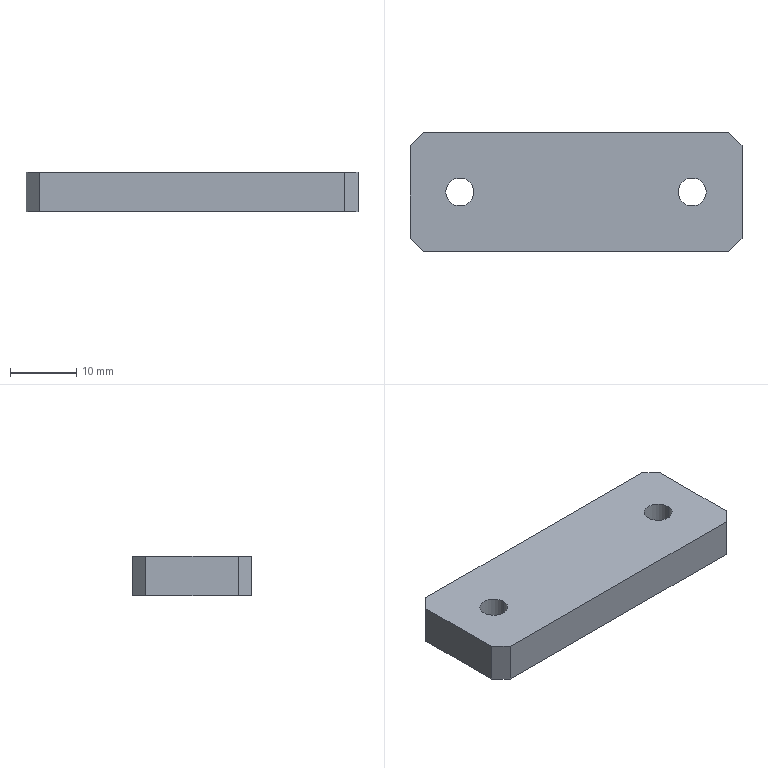Part | SolidWorks | features Chamfer 1, Extrusion 1, HoleWzd 1 | 1 solid | 14 faces | box 50 x 18 x 6 mm | volume 5186 mm3 | plane 10 | cylinder 4 | commonest cylinder face diameters 4.2 x4
STEP:
#1=CARTESIAN_POINT('',(-19.6,0.,-3.));
#2=VERTEX_POINT('',#1);
#3=CARTESIAN_POINT('',(-15.4,0.,-3.));
#4=VERTEX_POINT('',#3);
#5=CARTESIAN_POINT('',(-17.5,0.,-3.));
#6=DIRECTION('',(0.,0.,1.));
#7=DIRECTION('',(1.,0.,0.));
#8=AXIS2_PLACEMENT_3D('',#5,#6,#7);
#9=CIRCLE('',#8,2.1);
#10=EDGE_CURVE('',#2,#4,#9,.T.);
#11=ORIENTED_EDGE('',*,*,#10,.F.);
#12=CARTESIAN_POINT('',(-19.6,0.,3.));
#13=VERTEX_POINT('',#12);
#14=CARTESIAN_POINT('',(-19.6,0.,3.));
#15=DIRECTION('',(0.,0.,1.));
#16=VECTOR('',#15,1000.);
#17=LINE('',#14,#16);
#18=EDGE_CURVE('',#2,#13,#17,.T.);
#19=ORIENTED_EDGE('',*,*,#18,.T.);
#20=CARTESIAN_POINT('',(-15.4,0.,3.));
#21=VERTEX_POINT('',#20);
#22=CARTESIAN_POINT('',(-17.5,0.,3.));
#23=DIRECTION('',(0.,0.,1.));
#24=DIRECTION('',(1.,0.,0.));
#25=AXIS2_PLACEMENT_3D('',#22,#23,#24);
#26=CIRCLE('',#25,2.1);
#27=EDGE_CURVE('',#13,#21,#26,.T.);
#28=ORIENTED_EDGE('',*,*,#27,.T.);
#29=CARTESIAN_POINT('',(-15.4,0.,3.));
#30=DIRECTION('',(0.,0.,1.));
#31=VECTOR('',#30,1000.);
#32=LINE('',#29,#31);
#33=EDGE_CURVE('',#4,#21,#32,.T.);
#34=ORIENTED_EDGE('',*,*,#33,.F.);
#35=EDGE_LOOP('',(#11,#19,#28,#34));
#36=FACE_OUTER_BOUND('',#35,.T.);
#37=CARTESIAN_POINT('',(-17.5,0.,3.));
#38=DIRECTION('',(0.,0.,1.));
#39=DIRECTION('',(1.,0.,0.));
#40=AXIS2_PLACEMENT_3D('',#37,#38,#39);
#41=CYLINDRICAL_SURFACE('',#40,2.1);
#42=ADVANCED_FACE('',(#36),#41,.F.);
#43=CARTESIAN_POINT('',(15.4,0.,-3.));
#44=VERTEX_POINT('',#43);
#45=CARTESIAN_POINT('',(19.6,0.,-3.));
#46=VERTEX_POINT('',#45);
#47=CARTESIAN_POINT('',(17.5,0.,-3.));
#48=DIRECTION('',(0.,0.,1.));
#49=DIRECTION('',(1.,0.,0.));
#50=AXIS2_PLACEMENT_3D('',#47,#48,#49);
#51=CIRCLE('',#50,2.1);
#52=EDGE_CURVE('',#44,#46,#51,.T.);
#53=ORIENTED_EDGE('',*,*,#52,.F.);
#54=CARTESIAN_POINT('',(15.4,0.,3.));
#55=VERTEX_POINT('',#54);
#56=CARTESIAN_POINT('',(15.4,0.,3.));
#57=DIRECTION('',(0.,0.,1.));
#58=VECTOR('',#57,1000.);
#59=LINE('',#56,#58);
#60=EDGE_CURVE('',#44,#55,#59,.T.);
#61=ORIENTED_EDGE('',*,*,#60,.T.);
#62=CARTESIAN_POINT('',(19.6,0.,3.));
#63=VERTEX_POINT('',#62);
#64=CARTESIAN_POINT('',(17.5,0.,3.));
#65=DIRECTION('',(0.,0.,1.));
#66=DIRECTION('',(1.,0.,0.));
#67=AXIS2_PLACEMENT_3D('',#64,#65,#66);
#68=CIRCLE('',#67,2.1);
#69=EDGE_CURVE('',#55,#63,#68,.T.);
#70=ORIENTED_EDGE('',*,*,#69,.T.);
#71=CARTESIAN_POINT('',(19.6,0.,3.));
#72=DIRECTION('',(0.,0.,1.));
#73=VECTOR('',#72,1000.);
#74=LINE('',#71,#73);
#75=EDGE_CURVE('',#46,#63,#74,.T.);
#76=ORIENTED_EDGE('',*,*,#75,.F.);
#77=EDGE_LOOP('',(#53,#61,#70,#76));
#78=FACE_OUTER_BOUND('',#77,.T.);
#79=CARTESIAN_POINT('',(17.5,0.,3.));
#80=DIRECTION('',(0.,0.,1.));
#81=DIRECTION('',(1.,0.,0.));
#82=AXIS2_PLACEMENT_3D('',#79,#80,#81);
#83=CYLINDRICAL_SURFACE('',#82,2.1);
#84=ADVANCED_FACE('',(#78),#83,.F.);
#85=CARTESIAN_POINT('',(-25.,7.,-3.));
#86=VERTEX_POINT('',#85);
#87=CARTESIAN_POINT('',(-25.,-7.,-3.));
#88=VERTEX_POINT('',#87);
#89=CARTESIAN_POINT('',(-25.,-9.,-3.));
#90=DIRECTION('',(0.,-1.,0.));
#91=VECTOR('',#90,1000.);
#92=LINE('',#89,#91);
#93=EDGE_CURVE('',#86,#88,#92,.T.);
#94=ORIENTED_EDGE('',*,*,#93,.T.);
#95=CARTESIAN_POINT('',(-25.,-7.,3.));
#96=VERTEX_POINT('',#95);
#97=CARTESIAN_POINT('',(-25.,-7.,3.));
#98=DIRECTION('',(0.,0.,1.));
#99=VECTOR('',#98,1000.);
#100=LINE('',#97,#99);
#101=EDGE_CURVE('',#88,#96,#100,.T.);
#102=ORIENTED_EDGE('',*,*,#101,.T.);
#103=CARTESIAN_POINT('',(-25.,7.,3.));
#104=VERTEX_POINT('',#103);
#105=CARTESIAN_POINT('',(-25.,-9.,3.));
#106=DIRECTION('',(0.,-1.,0.));
#107=VECTOR('',#106,1000.);
#108=LINE('',#105,#107);
#109=EDGE_CURVE('',#104,#96,#108,.T.);
#110=ORIENTED_EDGE('',*,*,#109,.F.);
#111=CARTESIAN_POINT('',(-25.,7.,3.));
#112=DIRECTION('',(0.,0.,-1.));
#113=VECTOR('',#112,1000.);
#114=LINE('',#111,#113);
#115=EDGE_CURVE('',#104,#86,#114,.T.);
#116=ORIENTED_EDGE('',*,*,#115,.T.);
#117=EDGE_LOOP('',(#94,#102,#110,#116));
#118=FACE_OUTER_BOUND('',#117,.T.);
#119=CARTESIAN_POINT('',(-25.,-9.,3.));
#120=DIRECTION('',(1.,0.,0.));
#121=DIRECTION('',(0.,0.,-1.));
#122=AXIS2_PLACEMENT_3D('',#119,#120,#121);
#123=PLANE('',#122);
#124=ADVANCED_FACE('',(#118),#123,.F.);
#125=CARTESIAN_POINT('',(-23.,-9.,-3.));
#126=VERTEX_POINT('',#125);
#127=CARTESIAN_POINT('',(23.,-9.,-3.));
#128=VERTEX_POINT('',#127);
#129=CARTESIAN_POINT('',(25.,-9.,-3.));
#130=DIRECTION('',(1.,0.,0.));
#131=VECTOR('',#130,1000.);
#132=LINE('',#129,#131);
#133=EDGE_CURVE('',#126,#128,#132,.T.);
#134=ORIENTED_EDGE('',*,*,#133,.T.);
#135=CARTESIAN_POINT('',(23.,-9.,3.));
#136=VERTEX_POINT('',#135);
#137=CARTESIAN_POINT('',(23.,-9.,3.));
#138=DIRECTION('',(0.,0.,1.));
#139=VECTOR('',#138,1000.);
#140=LINE('',#137,#139);
#141=EDGE_CURVE('',#128,#136,#140,.T.);
#142=ORIENTED_EDGE('',*,*,#141,.T.);
#143=CARTESIAN_POINT('',(-23.,-9.,3.));
#144=VERTEX_POINT('',#143);
#145=CARTESIAN_POINT('',(25.,-9.,3.));
#146=DIRECTION('',(1.,0.,0.));
#147=VECTOR('',#146,1000.);
#148=LINE('',#145,#147);
#149=EDGE_CURVE('',#144,#136,#148,.T.);
#150=ORIENTED_EDGE('',*,*,#149,.F.);
#151=CARTESIAN_POINT('',(-23.,-9.,3.));
#152=DIRECTION('',(0.,0.,-1.));
#153=VECTOR('',#152,1000.);
#154=LINE('',#151,#153);
#155=EDGE_CURVE('',#144,#126,#154,.T.);
#156=ORIENTED_EDGE('',*,*,#155,.T.);
#157=EDGE_LOOP('',(#134,#142,#150,#156));
#158=FACE_OUTER_BOUND('',#157,.T.);
#159=CARTESIAN_POINT('',(25.,-9.,3.));
#160=DIRECTION('',(0.,1.,0.));
#161=DIRECTION('',(-1.,0.,0.));
#162=AXIS2_PLACEMENT_3D('',#159,#160,#161);
#163=PLANE('',#162);
#164=ADVANCED_FACE('',(#158),#163,.F.);
#165=CARTESIAN_POINT('',(25.,-7.,-3.));
#166=VERTEX_POINT('',#165);
#167=CARTESIAN_POINT('',(25.,7.,-3.));
#168=VERTEX_POINT('',#167);
#169=CARTESIAN_POINT('',(25.,-9.,-3.));
#170=DIRECTION('',(0.,1.,0.));
#171=VECTOR('',#170,1000.);
#172=LINE('',#169,#171);
#173=EDGE_CURVE('',#166,#168,#172,.T.);
#174=ORIENTED_EDGE('',*,*,#173,.T.);
#175=CARTESIAN_POINT('',(25.,7.,3.));
#176=VERTEX_POINT('',#175);
#177=CARTESIAN_POINT('',(25.,7.,3.));
#178=DIRECTION('',(0.,0.,1.));
#179=VECTOR('',#178,1000.);
#180=LINE('',#177,#179);
#181=EDGE_CURVE('',#168,#176,#180,.T.);
#182=ORIENTED_EDGE('',*,*,#181,.T.);
#183=CARTESIAN_POINT('',(25.,-7.,3.));
#184=VERTEX_POINT('',#183);
#185=CARTESIAN_POINT('',(25.,-9.,3.));
#186=DIRECTION('',(0.,1.,0.));
#187=VECTOR('',#186,1000.);
#188=LINE('',#185,#187);
#189=EDGE_CURVE('',#184,#176,#188,.T.);
#190=ORIENTED_EDGE('',*,*,#189,.F.);
#191=CARTESIAN_POINT('',(25.,-7.,3.));
#192=DIRECTION('',(0.,0.,-1.));
#193=VECTOR('',#192,1000.);
#194=LINE('',#191,#193);
#195=EDGE_CURVE('',#184,#166,#194,.T.);
#196=ORIENTED_EDGE('',*,*,#195,.T.);
#197=EDGE_LOOP('',(#174,#182,#190,#196));
#198=FACE_OUTER_BOUND('',#197,.T.);
#199=CARTESIAN_POINT('',(25.,-9.,3.));
#200=DIRECTION('',(-1.,0.,0.));
#201=DIRECTION('',(0.,0.,1.));
#202=AXIS2_PLACEMENT_3D('',#199,#200,#201);
#203=PLANE('',#202);
#204=ADVANCED_FACE('',(#198),#203,.F.);
#205=CARTESIAN_POINT('',(23.,9.,3.));
#206=VERTEX_POINT('',#205);
#207=CARTESIAN_POINT('',(-23.,9.,3.));
#208=VERTEX_POINT('',#207);
#209=CARTESIAN_POINT('',(25.,9.,3.));
#210=DIRECTION('',(-1.,0.,0.));
#211=VECTOR('',#210,1000.);
#212=LINE('',#209,#211);
#213=EDGE_CURVE('',#206,#208,#212,.T.);
#214=ORIENTED_EDGE('',*,*,#213,.F.);
#215=CARTESIAN_POINT('',(23.,9.,-3.));
#216=VERTEX_POINT('',#215);
#217=CARTESIAN_POINT('',(23.,9.,3.));
#218=DIRECTION('',(0.,0.,-1.));
#219=VECTOR('',#218,1000.);
#220=LINE('',#217,#219);
#221=EDGE_CURVE('',#206,#216,#220,.T.);
#222=ORIENTED_EDGE('',*,*,#221,.T.);
#223=CARTESIAN_POINT('',(-23.,9.,-3.));
#224=VERTEX_POINT('',#223);
#225=CARTESIAN_POINT('',(25.,9.,-3.));
#226=DIRECTION('',(-1.,0.,0.));
#227=VECTOR('',#226,1000.);
#228=LINE('',#225,#227);
#229=EDGE_CURVE('',#216,#224,#228,.T.);
#230=ORIENTED_EDGE('',*,*,#229,.T.);
#231=CARTESIAN_POINT('',(-23.,9.,3.));
#232=DIRECTION('',(0.,0.,1.));
#233=VECTOR('',#232,1000.);
#234=LINE('',#231,#233);
#235=EDGE_CURVE('',#224,#208,#234,.T.);
#236=ORIENTED_EDGE('',*,*,#235,.T.);
#237=EDGE_LOOP('',(#214,#222,#230,#236));
#238=FACE_OUTER_BOUND('',#237,.T.);
#239=CARTESIAN_POINT('',(25.,9.,3.));
#240=DIRECTION('',(0.,-1.,0.));
#241=DIRECTION('',(1.,0.,0.));
#242=AXIS2_PLACEMENT_3D('',#239,#240,#241);
#243=PLANE('',#242);
#244=ADVANCED_FACE('',(#238),#243,.F.);
#245=CARTESIAN_POINT('',(-17.5,0.,3.));
#246=DIRECTION('',(0.,0.,1.));
#247=DIRECTION('',(1.,0.,0.));
#248=AXIS2_PLACEMENT_3D('',#245,#246,#247);
#249=CIRCLE('',#248,2.1);
#250=EDGE_CURVE('',#21,#13,#249,.T.);
#251=ORIENTED_EDGE('',*,*,#250,.F.);
#252=ORIENTED_EDGE('',*,*,#27,.F.);
#253=EDGE_LOOP('',(#251,#252));
#254=FACE_BOUND('',#253,.T.);
#255=CARTESIAN_POINT('',(17.5,0.,3.));
#256=DIRECTION('',(0.,0.,1.));
#257=DIRECTION('',(1.,0.,0.));
#258=AXIS2_PLACEMENT_3D('',#255,#256,#257);
#259=CIRCLE('',#258,2.1);
#260=EDGE_CURVE('',#63,#55,#259,.T.);
#261=ORIENTED_EDGE('',*,*,#260,.F.);
#262=ORIENTED_EDGE('',*,*,#69,.F.);
#263=EDGE_LOOP('',(#261,#262));
#264=FACE_BOUND('',#263,.T.);
#265=ORIENTED_EDGE('',*,*,#189,.T.);
#266=CARTESIAN_POINT('',(16.,16.,3.));
#267=DIRECTION('',(-0.7071,0.7071,0.));
#268=VECTOR('',#267,1000.);
#269=LINE('',#266,#268);
#270=EDGE_CURVE('',#176,#206,#269,.T.);
#271=ORIENTED_EDGE('',*,*,#270,.T.);
#272=ORIENTED_EDGE('',*,*,#213,.T.);
#273=CARTESIAN_POINT('',(-16.,16.,3.));
#274=DIRECTION('',(-0.7071,-0.7071,0.));
#275=VECTOR('',#274,1000.);
#276=LINE('',#273,#275);
#277=EDGE_CURVE('',#208,#104,#276,.T.);
#278=ORIENTED_EDGE('',*,*,#277,.T.);
#279=ORIENTED_EDGE('',*,*,#109,.T.);
#280=CARTESIAN_POINT('',(-16.,-16.,3.));
#281=DIRECTION('',(0.7071,-0.7071,0.));
#282=VECTOR('',#281,1000.);
#283=LINE('',#280,#282);
#284=EDGE_CURVE('',#96,#144,#283,.T.);
#285=ORIENTED_EDGE('',*,*,#284,.T.);
#286=ORIENTED_EDGE('',*,*,#149,.T.);
#287=CARTESIAN_POINT('',(16.,-16.,3.));
#288=DIRECTION('',(0.7071,0.7071,0.));
#289=VECTOR('',#288,1000.);
#290=LINE('',#287,#289);
#291=EDGE_CURVE('',#136,#184,#290,.T.);
#292=ORIENTED_EDGE('',*,*,#291,.T.);
#293=EDGE_LOOP('',(#265,#271,#272,#278,#279,#285,#286,#292));
#294=FACE_OUTER_BOUND('',#293,.T.);
#295=CARTESIAN_POINT('',(0.,0.,3.));
#296=DIRECTION('',(0.,0.,1.));
#297=DIRECTION('',(1.,0.,0.));
#298=AXIS2_PLACEMENT_3D('',#295,#296,#297);
#299=PLANE('',#298);
#300=ADVANCED_FACE('',(#254,#264,#294),#299,.T.);
#301=CARTESIAN_POINT('',(-17.5,0.,-3.));
#302=DIRECTION('',(0.,0.,1.));
#303=DIRECTION('',(1.,0.,0.));
#304=AXIS2_PLACEMENT_3D('',#301,#302,#303);
#305=CIRCLE('',#304,2.1);
#306=EDGE_CURVE('',#4,#2,#305,.T.);
#307=ORIENTED_EDGE('',*,*,#306,.T.);
#308=ORIENTED_EDGE('',*,*,#10,.T.);
#309=EDGE_LOOP('',(#307,#308));
#310=FACE_BOUND('',#309,.T.);
#311=CARTESIAN_POINT('',(17.5,0.,-3.));
#312=DIRECTION('',(0.,0.,1.));
#313=DIRECTION('',(1.,0.,0.));
#314=AXIS2_PLACEMENT_3D('',#311,#312,#313);
#315=CIRCLE('',#314,2.1);
#316=EDGE_CURVE('',#46,#44,#315,.T.);
#317=ORIENTED_EDGE('',*,*,#316,.T.);
#318=ORIENTED_EDGE('',*,*,#52,.T.);
#319=EDGE_LOOP('',(#317,#318));
#320=FACE_BOUND('',#319,.T.);
#321=ORIENTED_EDGE('',*,*,#229,.F.);
#322=CARTESIAN_POINT('',(23.,9.,-3.));
#323=DIRECTION('',(0.7071,-0.7071,0.));
#324=VECTOR('',#323,1000.);
#325=LINE('',#322,#324);
#326=EDGE_CURVE('',#216,#168,#325,.T.);
#327=ORIENTED_EDGE('',*,*,#326,.T.);
#328=ORIENTED_EDGE('',*,*,#173,.F.);
#329=CARTESIAN_POINT('',(25.,-7.,-3.));
#330=DIRECTION('',(-0.7071,-0.7071,0.));
#331=VECTOR('',#330,1000.);
#332=LINE('',#329,#331);
#333=EDGE_CURVE('',#166,#128,#332,.T.);
#334=ORIENTED_EDGE('',*,*,#333,.T.);
#335=ORIENTED_EDGE('',*,*,#133,.F.);
#336=CARTESIAN_POINT('',(-23.,-9.,-3.));
#337=DIRECTION('',(-0.7071,0.7071,0.));
#338=VECTOR('',#337,1000.);
#339=LINE('',#336,#338);
#340=EDGE_CURVE('',#126,#88,#339,.T.);
#341=ORIENTED_EDGE('',*,*,#340,.T.);
#342=ORIENTED_EDGE('',*,*,#93,.F.);
#343=CARTESIAN_POINT('',(-25.,7.,-3.));
#344=DIRECTION('',(0.7071,0.7071,0.));
#345=VECTOR('',#344,1000.);
#346=LINE('',#343,#345);
#347=EDGE_CURVE('',#86,#224,#346,.T.);
#348=ORIENTED_EDGE('',*,*,#347,.T.);
#349=EDGE_LOOP('',(#321,#327,#328,#334,#335,#341,#342,#348));
#350=FACE_OUTER_BOUND('',#349,.T.);
#351=CARTESIAN_POINT('',(0.,0.,-3.));
#352=DIRECTION('',(0.,0.,1.));
#353=DIRECTION('',(1.,0.,0.));
#354=AXIS2_PLACEMENT_3D('',#351,#352,#353);
#355=PLANE('',#354);
#356=ADVANCED_FACE('',(#310,#320,#350),#355,.F.);
#357=ORIENTED_EDGE('',*,*,#60,.F.);
#358=ORIENTED_EDGE('',*,*,#316,.F.);
#359=ORIENTED_EDGE('',*,*,#75,.T.);
#360=ORIENTED_EDGE('',*,*,#260,.T.);
#361=EDGE_LOOP('',(#357,#358,#359,#360));
#362=FACE_OUTER_BOUND('',#361,.T.);
#363=CARTESIAN_POINT('',(17.5,0.,3.));
#364=DIRECTION('',(0.,0.,1.));
#365=DIRECTION('',(1.,0.,0.));
#366=AXIS2_PLACEMENT_3D('',#363,#364,#365);
#367=CYLINDRICAL_SURFACE('',#366,2.1);
#368=ADVANCED_FACE('',(#362),#367,.F.);
#369=ORIENTED_EDGE('',*,*,#18,.F.);
#370=ORIENTED_EDGE('',*,*,#306,.F.);
#371=ORIENTED_EDGE('',*,*,#33,.T.);
#372=ORIENTED_EDGE('',*,*,#250,.T.);
#373=EDGE_LOOP('',(#369,#370,#371,#372));
#374=FACE_OUTER_BOUND('',#373,.T.);
#375=CARTESIAN_POINT('',(-17.5,0.,3.));
#376=DIRECTION('',(0.,0.,1.));
#377=DIRECTION('',(1.,0.,0.));
#378=AXIS2_PLACEMENT_3D('',#375,#376,#377);
#379=CYLINDRICAL_SURFACE('',#378,2.1);
#380=ADVANCED_FACE('',(#374),#379,.F.);
#381=ORIENTED_EDGE('',*,*,#270,.F.);
#382=ORIENTED_EDGE('',*,*,#181,.F.);
#383=ORIENTED_EDGE('',*,*,#326,.F.);
#384=ORIENTED_EDGE('',*,*,#221,.F.);
#385=EDGE_LOOP('',(#381,#382,#383,#384));
#386=FACE_OUTER_BOUND('',#385,.T.);
#387=CARTESIAN_POINT('',(23.,9.,3.));
#388=DIRECTION('',(-0.7071,-0.7071,0.));
#389=DIRECTION('',(0.,0.,-1.));
#390=AXIS2_PLACEMENT_3D('',#387,#388,#389);
#391=PLANE('',#390);
#392=ADVANCED_FACE('',(#386),#391,.F.);
#393=ORIENTED_EDGE('',*,*,#291,.F.);
#394=ORIENTED_EDGE('',*,*,#141,.F.);
#395=ORIENTED_EDGE('',*,*,#333,.F.);
#396=ORIENTED_EDGE('',*,*,#195,.F.);
#397=EDGE_LOOP('',(#393,#394,#395,#396));
#398=FACE_OUTER_BOUND('',#397,.T.);
#399=CARTESIAN_POINT('',(25.,-7.,3.));
#400=DIRECTION('',(-0.7071,0.7071,0.));
#401=DIRECTION('',(0.,0.,-1.));
#402=AXIS2_PLACEMENT_3D('',#399,#400,#401);
#403=PLANE('',#402);
#404=ADVANCED_FACE('',(#398),#403,.F.);
#405=ORIENTED_EDGE('',*,*,#284,.F.);
#406=ORIENTED_EDGE('',*,*,#101,.F.);
#407=ORIENTED_EDGE('',*,*,#340,.F.);
#408=ORIENTED_EDGE('',*,*,#155,.F.);
#409=EDGE_LOOP('',(#405,#406,#407,#408));
#410=FACE_OUTER_BOUND('',#409,.T.);
#411=CARTESIAN_POINT('',(-23.,-9.,3.));
#412=DIRECTION('',(0.7071,0.7071,0.));
#413=DIRECTION('',(0.,0.,-1.));
#414=AXIS2_PLACEMENT_3D('',#411,#412,#413);
#415=PLANE('',#414);
#416=ADVANCED_FACE('',(#410),#415,.F.);
#417=ORIENTED_EDGE('',*,*,#277,.F.);
#418=ORIENTED_EDGE('',*,*,#235,.F.);
#419=ORIENTED_EDGE('',*,*,#347,.F.);
#420=ORIENTED_EDGE('',*,*,#115,.F.);
#421=EDGE_LOOP('',(#417,#418,#419,#420));
#422=FACE_OUTER_BOUND('',#421,.T.);
#423=CARTESIAN_POINT('',(-25.,7.,3.));
#424=DIRECTION('',(0.7071,-0.7071,0.));
#425=DIRECTION('',(0.,0.,-1.));
#426=AXIS2_PLACEMENT_3D('',#423,#424,#425);
#427=PLANE('',#426);
#428=ADVANCED_FACE('',(#422),#427,.F.);
#429=CLOSED_SHELL('',(#42,#84,#124,#164,#204,#244,#300,#356,#368,#380,#392,#404,#416,#428));
#430=MANIFOLD_SOLID_BREP('',#429);
#431=CARTESIAN_POINT('',(0.,0.,0.));
#432=DIRECTION('',(0.,0.,1.));
#433=DIRECTION('',(1.,0.,0.));
#434=AXIS2_PLACEMENT_3D('',#431,#432,#433);
#435=(LENGTH_UNIT()NAMED_UNIT(*)SI_UNIT(.MILLI.,.METRE.));
#436=UNCERTAINTY_MEASURE_WITH_UNIT(LENGTH_MEASURE(0.00001),#435,'','');
#437=(NAMED_UNIT(*)PLANE_ANGLE_UNIT()SI_UNIT($,.RADIAN.));
#438=(NAMED_UNIT(*)SI_UNIT($,.STERADIAN.)SOLID_ANGLE_UNIT());
#439=(GEOMETRIC_REPRESENTATION_CONTEXT(3)GLOBAL_UNCERTAINTY_ASSIGNED_CONTEXT((#436))GLOBAL_UNIT_ASSIGNED_CONTEXT((#435,#437,#438))REPRESENTATION_CONTEXT('',''));
#440=ADVANCED_BREP_SHAPE_REPRESENTATION('',(#430,#434),#439);